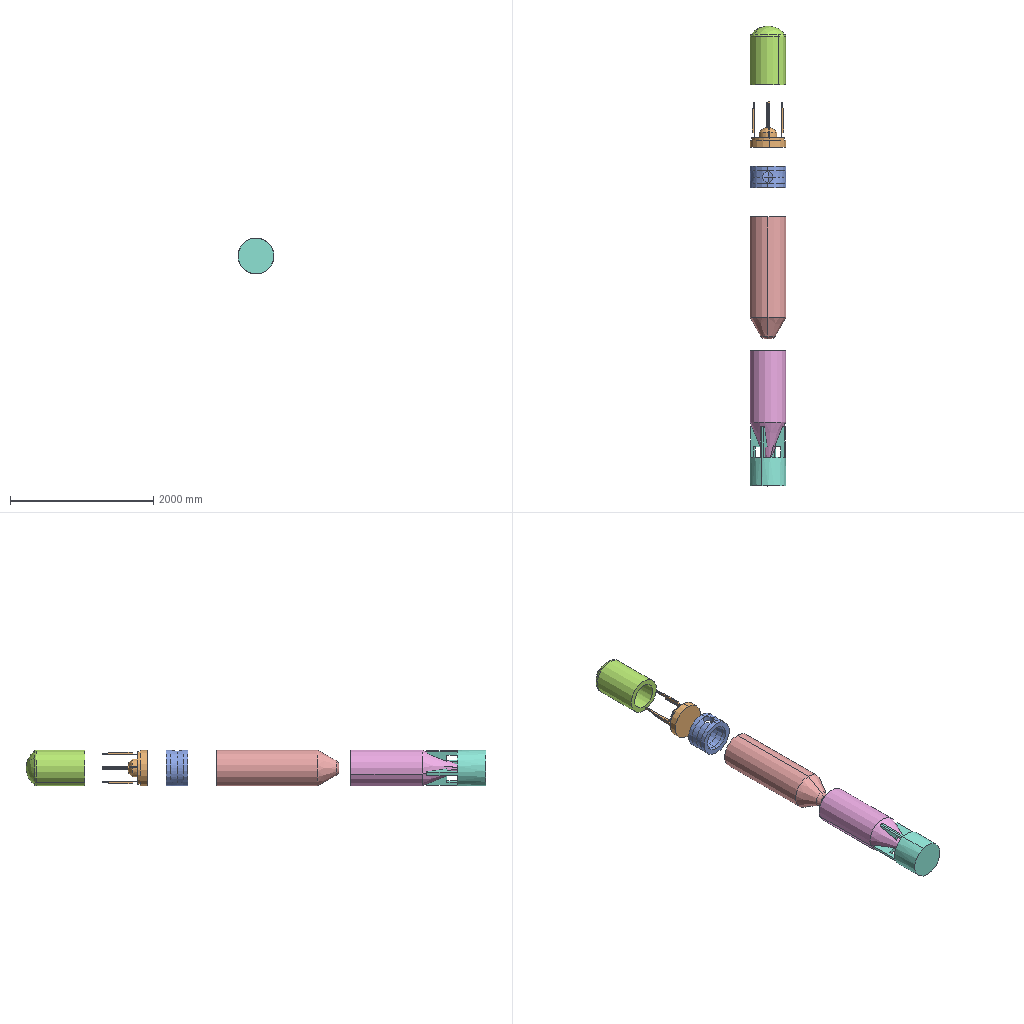Assembly | SolidWorks | 5 different items | 5 placed | box 500 x 6412 x 500 mm
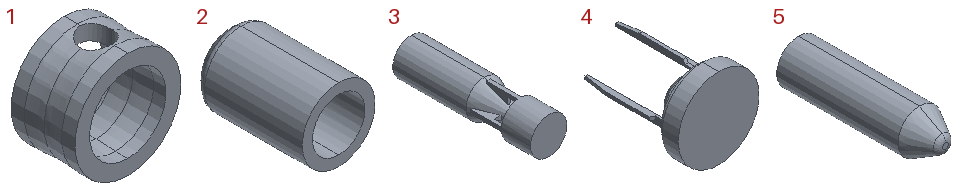Parts list (item | quantity | size | volume | features):
1 | x1 | 500 x 300 x 500 mm | 26874622 mm3 | features ICE 1, Revolution 1, Shell 1
2 | x1 | 500 x 820 x 500 mm | 76793679 mm3 | features Fillet 1, Revolution 1, Shell 1
3 | x1 | 500 x 1885 x 500 mm | 205239805 mm3 | features ICE 3, Revolution 2, Shell 1
4 | x1 | 500 x 630 x 500 mm | 31254702 mm3 | features ICE 3, Revolution 2, CirPattern 1
5 | x1 | 500 x 1700 x 500 mm | 151362883 mm3 | features Fillet 1, Revolution 1, Shell 1
Mates (type | each side: item.copy, entity, surface, feature):
Concentric | 5.1 face cylinder Revolve1 | 1.1 face cylinder Revolve1
Concentric | 1.1 face cylinder Revolve1 | 2.1 face cylinder Revolve1
Concentric | 5.1 face cylinder Revolve1 | 3.1 face cylinder Revolve1
Concentric | 1.1 face cylinder Revolve1 | 4.1 face cylinder Revolve1